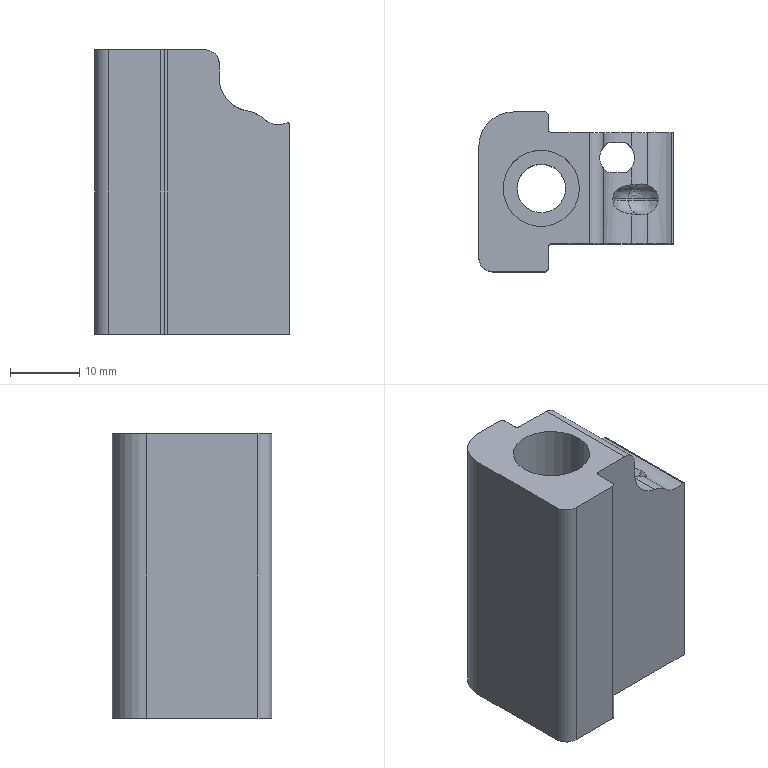Part | 1 solid | 44 faces | box 28 x 23 x 40.95 mm | volume 16406 mm3 | cylinder 21 | plane 17 | spline 6 | commonest cylinder face diameters 1 x4 4 x2 5 x2 7 x2 8.2 x2 9.5 x2